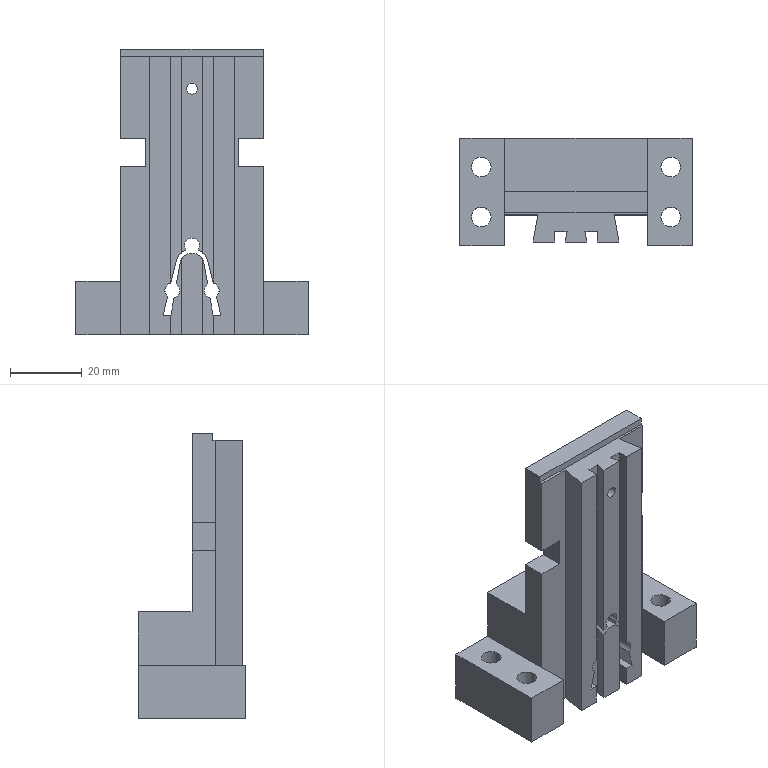Part | STEP file | slide seat 2 | 1 solid | 80 faces | box 65 x 30 x 80 mm | volume 57005 mm3 | plane 56 | cylinder 22 | cone 2 | commonest cylinder face diameters 5.5 x10 4.2 x5 2.5 x2 3 x2 9.2 x2 6.8 x1